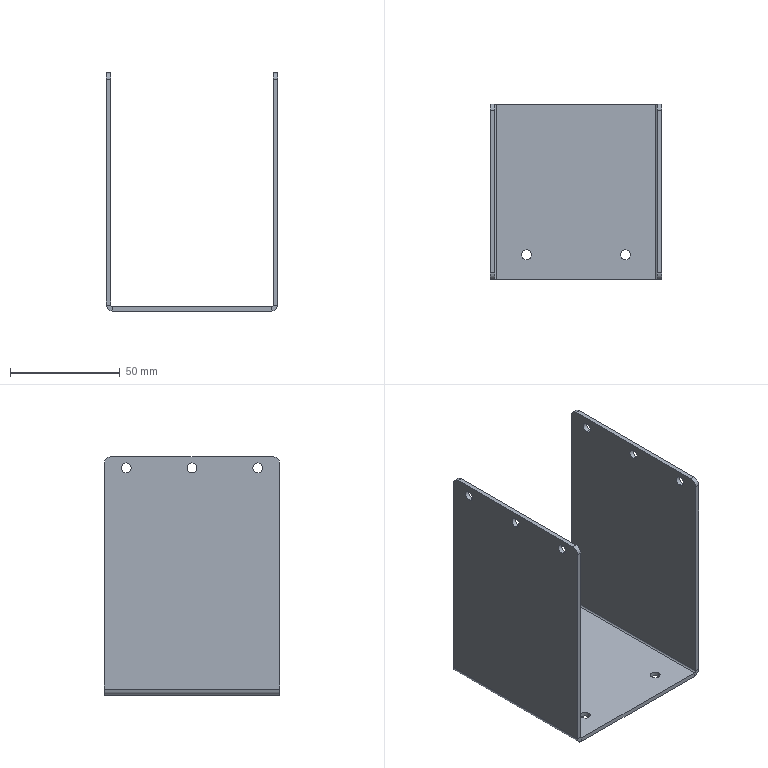Part | SolidWorks | features HoleWzd 2, Fillet 1, FlatPattern 1, SMBaseFlange 1, SheetMetal 1 | 1 solid | 42 faces | box 78 x 80 x 108.5 mm | volume 46050 mm3 | cylinder 24 | plane 18 | commonest cylinder face diameters 4.5 x16 6 x4 1.5 x2 5.5 x2
STEP:
#1=CARTESIAN_POINT('',(78.,10.,-7.25));
#2=VERTEX_POINT('',#1);
#3=CARTESIAN_POINT('',(78.,10.,-2.75));
#4=VERTEX_POINT('',#3);
#5=CARTESIAN_POINT('',(78.,10.,-5.));
#6=DIRECTION('',(-1.,0.,0.));
#7=DIRECTION('',(0.,0.,1.));
#8=AXIS2_PLACEMENT_3D('',#5,#6,#7);
#9=CIRCLE('',#8,2.25);
#10=EDGE_CURVE('',#2,#4,#9,.T.);
#11=ORIENTED_EDGE('',*,*,#10,.F.);
#12=CARTESIAN_POINT('',(76.,10.,-7.25));
#13=VERTEX_POINT('',#12);
#14=CARTESIAN_POINT('',(0.,10.,-7.25));
#15=DIRECTION('',(-1.,0.,0.));
#16=VECTOR('',#15,1000.);
#17=LINE('',#14,#16);
#18=EDGE_CURVE('',#2,#13,#17,.T.);
#19=ORIENTED_EDGE('',*,*,#18,.T.);
#20=CARTESIAN_POINT('',(76.,10.,-2.75));
#21=VERTEX_POINT('',#20);
#22=CARTESIAN_POINT('',(76.,10.,-5.));
#23=DIRECTION('',(1.,0.,0.));
#24=DIRECTION('',(0.,0.,-1.));
#25=AXIS2_PLACEMENT_3D('',#22,#23,#24);
#26=CIRCLE('',#25,2.25);
#27=EDGE_CURVE('',#21,#13,#26,.T.);
#28=ORIENTED_EDGE('',*,*,#27,.F.);
#29=CARTESIAN_POINT('',(0.,10.,-2.75));
#30=DIRECTION('',(-1.,0.,0.));
#31=VECTOR('',#30,1000.);
#32=LINE('',#29,#31);
#33=EDGE_CURVE('',#4,#21,#32,.T.);
#34=ORIENTED_EDGE('',*,*,#33,.F.);
#35=EDGE_LOOP('',(#11,#19,#28,#34));
#36=FACE_OUTER_BOUND('',#35,.T.);
#37=CARTESIAN_POINT('',(0.,10.,-5.));
#38=DIRECTION('',(-1.,0.,0.));
#39=DIRECTION('',(0.,0.,1.));
#40=AXIS2_PLACEMENT_3D('',#37,#38,#39);
#41=CYLINDRICAL_SURFACE('',#40,2.25);
#42=ADVANCED_FACE('',(#36),#41,.F.);
#43=CARTESIAN_POINT('',(2.,10.,-7.25));
#44=VERTEX_POINT('',#43);
#45=CARTESIAN_POINT('',(2.,10.,-2.75));
#46=VERTEX_POINT('',#45);
#47=CARTESIAN_POINT('',(2.,10.,-5.));
#48=DIRECTION('',(-1.,0.,0.));
#49=DIRECTION('',(0.,0.,1.));
#50=AXIS2_PLACEMENT_3D('',#47,#48,#49);
#51=CIRCLE('',#50,2.25);
#52=EDGE_CURVE('',#44,#46,#51,.T.);
#53=ORIENTED_EDGE('',*,*,#52,.F.);
#54=CARTESIAN_POINT('',(0.,10.,-7.25));
#55=VERTEX_POINT('',#54);
#56=CARTESIAN_POINT('',(0.,10.,-7.25));
#57=DIRECTION('',(-1.,0.,0.));
#58=VECTOR('',#57,1000.);
#59=LINE('',#56,#58);
#60=EDGE_CURVE('',#44,#55,#59,.T.);
#61=ORIENTED_EDGE('',*,*,#60,.T.);
#62=CARTESIAN_POINT('',(0.,10.,-2.75));
#63=VERTEX_POINT('',#62);
#64=CARTESIAN_POINT('',(0.,10.,-5.));
#65=DIRECTION('',(-1.,0.,0.));
#66=DIRECTION('',(0.,0.,1.));
#67=AXIS2_PLACEMENT_3D('',#64,#65,#66);
#68=CIRCLE('',#67,2.25);
#69=EDGE_CURVE('',#55,#63,#68,.T.);
#70=ORIENTED_EDGE('',*,*,#69,.T.);
#71=CARTESIAN_POINT('',(0.,10.,-2.75));
#72=DIRECTION('',(-1.,0.,0.));
#73=VECTOR('',#72,1000.);
#74=LINE('',#71,#73);
#75=EDGE_CURVE('',#46,#63,#74,.T.);
#76=ORIENTED_EDGE('',*,*,#75,.F.);
#77=EDGE_LOOP('',(#53,#61,#70,#76));
#78=FACE_OUTER_BOUND('',#77,.T.);
#79=CARTESIAN_POINT('',(0.,10.,-5.));
#80=DIRECTION('',(-1.,0.,0.));
#81=DIRECTION('',(0.,0.,1.));
#82=AXIS2_PLACEMENT_3D('',#79,#80,#81);
#83=CYLINDRICAL_SURFACE('',#82,2.25);
#84=ADVANCED_FACE('',(#78),#83,.F.);
#85=CARTESIAN_POINT('',(2.,40.,-7.25));
#86=VERTEX_POINT('',#85);
#87=CARTESIAN_POINT('',(2.,40.,-2.75));
#88=VERTEX_POINT('',#87);
#89=CARTESIAN_POINT('',(2.,40.,-5.));
#90=DIRECTION('',(-1.,0.,0.));
#91=DIRECTION('',(0.,0.,1.));
#92=AXIS2_PLACEMENT_3D('',#89,#90,#91);
#93=CIRCLE('',#92,2.25);
#94=EDGE_CURVE('',#86,#88,#93,.T.);
#95=ORIENTED_EDGE('',*,*,#94,.F.);
#96=CARTESIAN_POINT('',(0.,40.,-7.25));
#97=VERTEX_POINT('',#96);
#98=CARTESIAN_POINT('',(0.,40.,-7.25));
#99=DIRECTION('',(-1.,0.,0.));
#100=VECTOR('',#99,1000.);
#101=LINE('',#98,#100);
#102=EDGE_CURVE('',#86,#97,#101,.T.);
#103=ORIENTED_EDGE('',*,*,#102,.T.);
#104=CARTESIAN_POINT('',(0.,40.,-2.75));
#105=VERTEX_POINT('',#104);
#106=CARTESIAN_POINT('',(0.,40.,-5.));
#107=DIRECTION('',(-1.,0.,0.));
#108=DIRECTION('',(0.,0.,1.));
#109=AXIS2_PLACEMENT_3D('',#106,#107,#108);
#110=CIRCLE('',#109,2.25);
#111=EDGE_CURVE('',#97,#105,#110,.T.);
#112=ORIENTED_EDGE('',*,*,#111,.T.);
#113=CARTESIAN_POINT('',(0.,40.,-2.75));
#114=DIRECTION('',(-1.,0.,0.));
#115=VECTOR('',#114,1000.);
#116=LINE('',#113,#115);
#117=EDGE_CURVE('',#88,#105,#116,.T.);
#118=ORIENTED_EDGE('',*,*,#117,.F.);
#119=EDGE_LOOP('',(#95,#103,#112,#118));
#120=FACE_OUTER_BOUND('',#119,.T.);
#121=CARTESIAN_POINT('',(0.,40.,-5.));
#122=DIRECTION('',(-1.,0.,0.));
#123=DIRECTION('',(0.,0.,1.));
#124=AXIS2_PLACEMENT_3D('',#121,#122,#123);
#125=CYLINDRICAL_SURFACE('',#124,2.25);
#126=ADVANCED_FACE('',(#120),#125,.F.);
#127=CARTESIAN_POINT('',(78.,40.,-7.25));
#128=VERTEX_POINT('',#127);
#129=CARTESIAN_POINT('',(78.,40.,-2.75));
#130=VERTEX_POINT('',#129);
#131=CARTESIAN_POINT('',(78.,40.,-5.));
#132=DIRECTION('',(-1.,0.,0.));
#133=DIRECTION('',(0.,0.,1.));
#134=AXIS2_PLACEMENT_3D('',#131,#132,#133);
#135=CIRCLE('',#134,2.25);
#136=EDGE_CURVE('',#128,#130,#135,.T.);
#137=ORIENTED_EDGE('',*,*,#136,.F.);
#138=CARTESIAN_POINT('',(76.,40.,-7.25));
#139=VERTEX_POINT('',#138);
#140=CARTESIAN_POINT('',(0.,40.,-7.25));
#141=DIRECTION('',(-1.,0.,0.));
#142=VECTOR('',#141,1000.);
#143=LINE('',#140,#142);
#144=EDGE_CURVE('',#128,#139,#143,.T.);
#145=ORIENTED_EDGE('',*,*,#144,.T.);
#146=CARTESIAN_POINT('',(76.,40.,-2.75));
#147=VERTEX_POINT('',#146);
#148=CARTESIAN_POINT('',(76.,40.,-5.));
#149=DIRECTION('',(1.,0.,0.));
#150=DIRECTION('',(0.,0.,-1.));
#151=AXIS2_PLACEMENT_3D('',#148,#149,#150);
#152=CIRCLE('',#151,2.25);
#153=EDGE_CURVE('',#147,#139,#152,.T.);
#154=ORIENTED_EDGE('',*,*,#153,.F.);
#155=CARTESIAN_POINT('',(0.,40.,-2.75));
#156=DIRECTION('',(-1.,0.,0.));
#157=VECTOR('',#156,1000.);
#158=LINE('',#155,#157);
#159=EDGE_CURVE('',#130,#147,#158,.T.);
#160=ORIENTED_EDGE('',*,*,#159,.F.);
#161=EDGE_LOOP('',(#137,#145,#154,#160));
#162=FACE_OUTER_BOUND('',#161,.T.);
#163=CARTESIAN_POINT('',(0.,40.,-5.));
#164=DIRECTION('',(-1.,0.,0.));
#165=DIRECTION('',(0.,0.,1.));
#166=AXIS2_PLACEMENT_3D('',#163,#164,#165);
#167=CYLINDRICAL_SURFACE('',#166,2.25);
#168=ADVANCED_FACE('',(#162),#167,.F.);
#169=CARTESIAN_POINT('',(2.,70.,-7.25));
#170=VERTEX_POINT('',#169);
#171=CARTESIAN_POINT('',(2.,70.,-2.75));
#172=VERTEX_POINT('',#171);
#173=CARTESIAN_POINT('',(2.,70.,-5.));
#174=DIRECTION('',(-1.,0.,0.));
#175=DIRECTION('',(0.,0.,1.));
#176=AXIS2_PLACEMENT_3D('',#173,#174,#175);
#177=CIRCLE('',#176,2.25);
#178=EDGE_CURVE('',#170,#172,#177,.T.);
#179=ORIENTED_EDGE('',*,*,#178,.F.);
#180=CARTESIAN_POINT('',(0.,70.,-7.25));
#181=VERTEX_POINT('',#180);
#182=CARTESIAN_POINT('',(0.,70.,-7.25));
#183=DIRECTION('',(-1.,0.,0.));
#184=VECTOR('',#183,1000.);
#185=LINE('',#182,#184);
#186=EDGE_CURVE('',#170,#181,#185,.T.);
#187=ORIENTED_EDGE('',*,*,#186,.T.);
#188=CARTESIAN_POINT('',(0.,70.,-2.75));
#189=VERTEX_POINT('',#188);
#190=CARTESIAN_POINT('',(0.,70.,-5.));
#191=DIRECTION('',(-1.,0.,0.));
#192=DIRECTION('',(0.,0.,1.));
#193=AXIS2_PLACEMENT_3D('',#190,#191,#192);
#194=CIRCLE('',#193,2.25);
#195=EDGE_CURVE('',#181,#189,#194,.T.);
#196=ORIENTED_EDGE('',*,*,#195,.T.);
#197=CARTESIAN_POINT('',(0.,70.,-2.75));
#198=DIRECTION('',(-1.,0.,0.));
#199=VECTOR('',#198,1000.);
#200=LINE('',#197,#199);
#201=EDGE_CURVE('',#172,#189,#200,.T.);
#202=ORIENTED_EDGE('',*,*,#201,.F.);
#203=EDGE_LOOP('',(#179,#187,#196,#202));
#204=FACE_OUTER_BOUND('',#203,.T.);
#205=CARTESIAN_POINT('',(0.,70.,-5.));
#206=DIRECTION('',(-1.,0.,0.));
#207=DIRECTION('',(0.,0.,1.));
#208=AXIS2_PLACEMENT_3D('',#205,#206,#207);
#209=CYLINDRICAL_SURFACE('',#208,2.25);
#210=ADVANCED_FACE('',(#204),#209,.F.);
#211=CARTESIAN_POINT('',(78.,70.,-7.25));
#212=VERTEX_POINT('',#211);
#213=CARTESIAN_POINT('',(78.,70.,-2.75));
#214=VERTEX_POINT('',#213);
#215=CARTESIAN_POINT('',(78.,70.,-5.));
#216=DIRECTION('',(-1.,0.,0.));
#217=DIRECTION('',(0.,0.,1.));
#218=AXIS2_PLACEMENT_3D('',#215,#216,#217);
#219=CIRCLE('',#218,2.25);
#220=EDGE_CURVE('',#212,#214,#219,.T.);
#221=ORIENTED_EDGE('',*,*,#220,.F.);
#222=CARTESIAN_POINT('',(76.,70.,-7.25));
#223=VERTEX_POINT('',#222);
#224=CARTESIAN_POINT('',(0.,70.,-7.25));
#225=DIRECTION('',(-1.,0.,0.));
#226=VECTOR('',#225,1000.);
#227=LINE('',#224,#226);
#228=EDGE_CURVE('',#212,#223,#227,.T.);
#229=ORIENTED_EDGE('',*,*,#228,.T.);
#230=CARTESIAN_POINT('',(76.,70.,-2.75));
#231=VERTEX_POINT('',#230);
#232=CARTESIAN_POINT('',(76.,70.,-5.));
#233=DIRECTION('',(1.,0.,0.));
#234=DIRECTION('',(0.,0.,-1.));
#235=AXIS2_PLACEMENT_3D('',#232,#233,#234);
#236=CIRCLE('',#235,2.25);
#237=EDGE_CURVE('',#231,#223,#236,.T.);
#238=ORIENTED_EDGE('',*,*,#237,.F.);
#239=CARTESIAN_POINT('',(0.,70.,-2.75));
#240=DIRECTION('',(-1.,0.,0.));
#241=VECTOR('',#240,1000.);
#242=LINE('',#239,#241);
#243=EDGE_CURVE('',#214,#231,#242,.T.);
#244=ORIENTED_EDGE('',*,*,#243,.F.);
#245=EDGE_LOOP('',(#221,#229,#238,#244));
#246=FACE_OUTER_BOUND('',#245,.T.);
#247=CARTESIAN_POINT('',(0.,70.,-5.));
#248=DIRECTION('',(-1.,0.,0.));
#249=DIRECTION('',(0.,0.,1.));
#250=AXIS2_PLACEMENT_3D('',#247,#248,#249);
#251=CYLINDRICAL_SURFACE('',#250,2.25);
#252=ADVANCED_FACE('',(#246),#251,.F.);
#253=CARTESIAN_POINT('',(63.75,11.5,-106.5));
#254=VERTEX_POINT('',#253);
#255=CARTESIAN_POINT('',(59.25,11.5,-106.5));
#256=VERTEX_POINT('',#255);
#257=CARTESIAN_POINT('',(61.5,11.5,-106.5));
#258=DIRECTION('',(0.,0.,-1.));
#259=DIRECTION('',(-1.,0.,0.));
#260=AXIS2_PLACEMENT_3D('',#257,#258,#259);
#261=CIRCLE('',#260,2.25);
#262=EDGE_CURVE('',#254,#256,#261,.T.);
#263=ORIENTED_EDGE('',*,*,#262,.F.);
#264=CARTESIAN_POINT('',(63.75,11.5,-108.5));
#265=VERTEX_POINT('',#264);
#266=CARTESIAN_POINT('',(63.75,11.5,-108.5));
#267=DIRECTION('',(0.,0.,-1.));
#268=VECTOR('',#267,1000.);
#269=LINE('',#266,#268);
#270=EDGE_CURVE('',#254,#265,#269,.T.);
#271=ORIENTED_EDGE('',*,*,#270,.T.);
#272=CARTESIAN_POINT('',(59.25,11.5,-108.5));
#273=VERTEX_POINT('',#272);
#274=CARTESIAN_POINT('',(61.5,11.5,-108.5));
#275=DIRECTION('',(0.,0.,-1.));
#276=DIRECTION('',(-1.,0.,0.));
#277=AXIS2_PLACEMENT_3D('',#274,#275,#276);
#278=CIRCLE('',#277,2.25);
#279=EDGE_CURVE('',#265,#273,#278,.T.);
#280=ORIENTED_EDGE('',*,*,#279,.T.);
#281=CARTESIAN_POINT('',(59.25,11.5,-108.5));
#282=DIRECTION('',(0.,0.,-1.));
#283=VECTOR('',#282,1000.);
#284=LINE('',#281,#283);
#285=EDGE_CURVE('',#256,#273,#284,.T.);
#286=ORIENTED_EDGE('',*,*,#285,.F.);
#287=EDGE_LOOP('',(#263,#271,#280,#286));
#288=FACE_OUTER_BOUND('',#287,.T.);
#289=CARTESIAN_POINT('',(61.5,11.5,-108.5));
#290=DIRECTION('',(0.,0.,-1.));
#291=DIRECTION('',(-1.,0.,0.));
#292=AXIS2_PLACEMENT_3D('',#289,#290,#291);
#293=CYLINDRICAL_SURFACE('',#292,2.25);
#294=ADVANCED_FACE('',(#288),#293,.F.);
#295=CARTESIAN_POINT('',(18.75,11.5,-106.5));
#296=VERTEX_POINT('',#295);
#297=CARTESIAN_POINT('',(14.25,11.5,-106.5));
#298=VERTEX_POINT('',#297);
#299=CARTESIAN_POINT('',(16.5,11.5,-106.5));
#300=DIRECTION('',(0.,0.,-1.));
#301=DIRECTION('',(-1.,0.,0.));
#302=AXIS2_PLACEMENT_3D('',#299,#300,#301);
#303=CIRCLE('',#302,2.25);
#304=EDGE_CURVE('',#296,#298,#303,.T.);
#305=ORIENTED_EDGE('',*,*,#304,.F.);
#306=CARTESIAN_POINT('',(18.75,11.5,-108.5));
#307=VERTEX_POINT('',#306);
#308=CARTESIAN_POINT('',(18.75,11.5,-108.5));
#309=DIRECTION('',(0.,0.,-1.));
#310=VECTOR('',#309,1000.);
#311=LINE('',#308,#310);
#312=EDGE_CURVE('',#296,#307,#311,.T.);
#313=ORIENTED_EDGE('',*,*,#312,.T.);
#314=CARTESIAN_POINT('',(14.25,11.5,-108.5));
#315=VERTEX_POINT('',#314);
#316=CARTESIAN_POINT('',(16.5,11.5,-108.5));
#317=DIRECTION('',(0.,0.,-1.));
#318=DIRECTION('',(-1.,0.,0.));
#319=AXIS2_PLACEMENT_3D('',#316,#317,#318);
#320=CIRCLE('',#319,2.25);
#321=EDGE_CURVE('',#307,#315,#320,.T.);
#322=ORIENTED_EDGE('',*,*,#321,.T.);
#323=CARTESIAN_POINT('',(14.25,11.5,-108.5));
#324=DIRECTION('',(0.,0.,-1.));
#325=VECTOR('',#324,1000.);
#326=LINE('',#323,#325);
#327=EDGE_CURVE('',#298,#315,#326,.T.);
#328=ORIENTED_EDGE('',*,*,#327,.F.);
#329=EDGE_LOOP('',(#305,#313,#322,#328));
#330=FACE_OUTER_BOUND('',#329,.T.);
#331=CARTESIAN_POINT('',(16.5,11.5,-108.5));
#332=DIRECTION('',(0.,0.,-1.));
#333=DIRECTION('',(-1.,0.,0.));
#334=AXIS2_PLACEMENT_3D('',#331,#332,#333);
#335=CYLINDRICAL_SURFACE('',#334,2.25);
#336=ADVANCED_FACE('',(#330),#335,.F.);
#337=CARTESIAN_POINT('',(2.75,80.,-108.5));
#338=VERTEX_POINT('',#337);
#339=CARTESIAN_POINT('',(2.75,80.,-106.5));
#340=VERTEX_POINT('',#339);
#341=CARTESIAN_POINT('',(2.75,80.,-108.5));
#342=DIRECTION('',(0.,0.,1.));
#343=VECTOR('',#342,1000.);
#344=LINE('',#341,#343);
#345=EDGE_CURVE('',#338,#340,#344,.T.);
#346=ORIENTED_EDGE('',*,*,#345,.F.);
#347=CARTESIAN_POINT('',(0.,80.,-105.75));
#348=VERTEX_POINT('',#347);
#349=CARTESIAN_POINT('',(2.75,80.,-105.75));
#350=DIRECTION('',(0.,-1.,0.));
#351=DIRECTION('',(0.,0.,1.));
#352=AXIS2_PLACEMENT_3D('',#349,#350,#351);
#353=CIRCLE('',#352,2.75);
#354=EDGE_CURVE('',#348,#338,#353,.T.);
#355=ORIENTED_EDGE('',*,*,#354,.F.);
#356=CARTESIAN_POINT('',(2.,80.,-105.75));
#357=VERTEX_POINT('',#356);
#358=CARTESIAN_POINT('',(2.,80.,-105.75));
#359=DIRECTION('',(-1.,0.,0.));
#360=VECTOR('',#359,1000.);
#361=LINE('',#358,#360);
#362=EDGE_CURVE('',#357,#348,#361,.T.);
#363=ORIENTED_EDGE('',*,*,#362,.F.);
#364=CARTESIAN_POINT('',(2.75,80.,-105.75));
#365=DIRECTION('',(0.,-1.,0.));
#366=DIRECTION('',(1.,0.,0.));
#367=AXIS2_PLACEMENT_3D('',#364,#365,#366);
#368=CIRCLE('',#367,0.75);
#369=EDGE_CURVE('',#357,#340,#368,.T.);
#370=ORIENTED_EDGE('',*,*,#369,.T.);
#371=EDGE_LOOP('',(#346,#355,#363,#370));
#372=FACE_OUTER_BOUND('',#371,.T.);
#373=CARTESIAN_POINT('',(2.75,80.,-108.5));
#374=DIRECTION('',(0.,1.,0.));
#375=DIRECTION('',(0.,0.,1.));
#376=AXIS2_PLACEMENT_3D('',#373,#374,#375);
#377=PLANE('',#376);
#378=ADVANCED_FACE('',(#372),#377,.T.);
#379=CARTESIAN_POINT('',(75.25,80.,-108.5));
#380=VERTEX_POINT('',#379);
#381=CARTESIAN_POINT('',(0.,80.,-108.5));
#382=DIRECTION('',(1.,0.,0.));
#383=VECTOR('',#382,1000.);
#384=LINE('',#381,#383);
#385=EDGE_CURVE('',#338,#380,#384,.T.);
#386=ORIENTED_EDGE('',*,*,#385,.F.);
#387=ORIENTED_EDGE('',*,*,#345,.T.);
#388=CARTESIAN_POINT('',(75.25,80.,-106.5));
#389=VERTEX_POINT('',#388);
#390=CARTESIAN_POINT('',(0.,80.,-106.5));
#391=DIRECTION('',(1.,0.,0.));
#392=VECTOR('',#391,1000.);
#393=LINE('',#390,#392);
#394=EDGE_CURVE('',#340,#389,#393,.T.);
#395=ORIENTED_EDGE('',*,*,#394,.T.);
#396=CARTESIAN_POINT('',(75.25,80.,-106.5));
#397=DIRECTION('',(0.,0.,-1.));
#398=VECTOR('',#397,1000.);
#399=LINE('',#396,#398);
#400=EDGE_CURVE('',#389,#380,#399,.T.);
#401=ORIENTED_EDGE('',*,*,#400,.T.);
#402=EDGE_LOOP('',(#386,#387,#395,#401));
#403=FACE_OUTER_BOUND('',#402,.T.);
#404=CARTESIAN_POINT('',(2.,80.,-105.75));
#405=DIRECTION('',(0.,1.,0.));
#406=DIRECTION('',(0.,0.,1.));
#407=AXIS2_PLACEMENT_3D('',#404,#405,#406);
#408=PLANE('',#407);
#409=ADVANCED_FACE('',(#403),#408,.T.);
#410=CARTESIAN_POINT('',(0.,0.,-105.75));
#411=VERTEX_POINT('',#410);
#412=CARTESIAN_POINT('',(2.,0.,-105.75));
#413=VERTEX_POINT('',#412);
#414=CARTESIAN_POINT('',(0.,0.,-105.75));
#415=DIRECTION('',(1.,0.,0.));
#416=VECTOR('',#415,1000.);
#417=LINE('',#414,#416);
#418=EDGE_CURVE('',#411,#413,#417,.T.);
#419=ORIENTED_EDGE('',*,*,#418,.F.);
#420=CARTESIAN_POINT('',(2.75,0.,-108.5));
#421=VERTEX_POINT('',#420);
#422=CARTESIAN_POINT('',(2.75,0.,-105.75));
#423=DIRECTION('',(0.,-1.,0.));
#424=DIRECTION('',(0.,0.,1.));
#425=AXIS2_PLACEMENT_3D('',#422,#423,#424);
#426=CIRCLE('',#425,2.75);
#427=EDGE_CURVE('',#411,#421,#426,.T.);
#428=ORIENTED_EDGE('',*,*,#427,.T.);
#429=CARTESIAN_POINT('',(2.75,0.,-106.5));
#430=VERTEX_POINT('',#429);
#431=CARTESIAN_POINT('',(2.75,0.,-106.5));
#432=DIRECTION('',(0.,0.,-1.));
#433=VECTOR('',#432,1000.);
#434=LINE('',#431,#433);
#435=EDGE_CURVE('',#430,#421,#434,.T.);
#436=ORIENTED_EDGE('',*,*,#435,.F.);
#437=CARTESIAN_POINT('',(2.75,0.,-105.75));
#438=DIRECTION('',(0.,-1.,0.));
#439=DIRECTION('',(1.,0.,0.));
#440=AXIS2_PLACEMENT_3D('',#437,#438,#439);
#441=CIRCLE('',#440,0.75);
#442=EDGE_CURVE('',#413,#430,#441,.T.);
#443=ORIENTED_EDGE('',*,*,#442,.F.);
#444=EDGE_LOOP('',(#419,#428,#436,#443));
#445=FACE_OUTER_BOUND('',#444,.T.);
#446=CARTESIAN_POINT('',(0.,0.,-105.75));
#447=DIRECTION('',(0.,-1.,0.));
#448=DIRECTION('',(0.,0.,-1.));
#449=AXIS2_PLACEMENT_3D('',#446,#447,#448);
#450=PLANE('',#449);
#451=ADVANCED_FACE('',(#445),#450,.T.);
#452=CARTESIAN_POINT('',(2.,0.,-3.));
#453=VERTEX_POINT('',#452);
#454=CARTESIAN_POINT('',(2.,0.,0.));
#455=DIRECTION('',(0.,0.,-1.));
#456=VECTOR('',#455,1000.);
#457=LINE('',#454,#456);
#458=EDGE_CURVE('',#453,#413,#457,.T.);
#459=ORIENTED_EDGE('',*,*,#458,.F.);
#460=CARTESIAN_POINT('',(0.,0.,-3.));
#461=VERTEX_POINT('',#460);
#462=CARTESIAN_POINT('',(2.75,0.,-3.));
#463=DIRECTION('',(-1.,0.,0.));
#464=VECTOR('',#463,1000.);
#465=LINE('',#462,#464);
#466=EDGE_CURVE('',#453,#461,#465,.T.);
#467=ORIENTED_EDGE('',*,*,#466,.T.);
#468=CARTESIAN_POINT('',(0.,0.,0.));
#469=DIRECTION('',(0.,0.,-1.));
#470=VECTOR('',#469,1000.);
#471=LINE('',#468,#470);
#472=EDGE_CURVE('',#461,#411,#471,.T.);
#473=ORIENTED_EDGE('',*,*,#472,.T.);
#474=ORIENTED_EDGE('',*,*,#418,.T.);
#475=EDGE_LOOP('',(#459,#467,#473,#474));
#476=FACE_OUTER_BOUND('',#475,.T.);
#477=CARTESIAN_POINT('',(2.75,0.,-106.5));
#478=DIRECTION('',(0.,-1.,0.));
#479=DIRECTION('',(0.,0.,-1.));
#480=AXIS2_PLACEMENT_3D('',#477,#478,#479);
#481=PLANE('',#480);
#482=ADVANCED_FACE('',(#476),#481,.T.);
#483=CARTESIAN_POINT('',(78.,80.,-105.75));
#484=VERTEX_POINT('',#483);
#485=CARTESIAN_POINT('',(76.,80.,-105.75));
#486=VERTEX_POINT('',#485);
#487=CARTESIAN_POINT('',(78.,80.,-105.75));
#488=DIRECTION('',(-1.,0.,0.));
#489=VECTOR('',#488,1000.);
#490=LINE('',#487,#489);
#491=EDGE_CURVE('',#484,#486,#490,.T.);
#492=ORIENTED_EDGE('',*,*,#491,.F.);
#493=CARTESIAN_POINT('',(75.25,80.,-105.75));
#494=DIRECTION('',(0.,-1.,0.));
#495=DIRECTION('',(0.,0.,1.));
#496=AXIS2_PLACEMENT_3D('',#493,#494,#495);
#497=CIRCLE('',#496,2.75);
#498=EDGE_CURVE('',#380,#484,#497,.T.);
#499=ORIENTED_EDGE('',*,*,#498,.F.);
#500=ORIENTED_EDGE('',*,*,#400,.F.);
#501=CARTESIAN_POINT('',(75.25,80.,-105.75));
#502=DIRECTION('',(0.,-1.,0.));
#503=DIRECTION('',(1.,0.,0.));
#504=AXIS2_PLACEMENT_3D('',#501,#502,#503);
#505=CIRCLE('',#504,0.75);
#506=EDGE_CURVE('',#389,#486,#505,.T.);
#507=ORIENTED_EDGE('',*,*,#506,.T.);
#508=EDGE_LOOP('',(#492,#499,#500,#507));
#509=FACE_OUTER_BOUND('',#508,.T.);
#510=CARTESIAN_POINT('',(78.,80.,-105.75));
#511=DIRECTION('',(0.,1.,0.));
#512=DIRECTION('',(0.,0.,1.));
#513=AXIS2_PLACEMENT_3D('',#510,#511,#512);
#514=PLANE('',#513);
#515=ADVANCED_FACE('',(#509),#514,.T.);
#516=CARTESIAN_POINT('',(76.,80.,-3.));
#517=VERTEX_POINT('',#516);
#518=CARTESIAN_POINT('',(76.,80.,-108.5));
#519=DIRECTION('',(0.,0.,1.));
#520=VECTOR('',#519,1000.);
#521=LINE('',#518,#520);
#522=EDGE_CURVE('',#486,#517,#521,.T.);
#523=ORIENTED_EDGE('',*,*,#522,.T.);
#524=CARTESIAN_POINT('',(78.,80.,-3.));
#525=VERTEX_POINT('',#524);
#526=CARTESIAN_POINT('',(75.25,80.,-3.));
#527=DIRECTION('',(1.,0.,0.));
#528=VECTOR('',#527,1000.);
#529=LINE('',#526,#528);
#530=EDGE_CURVE('',#517,#525,#529,.T.);
#531=ORIENTED_EDGE('',*,*,#530,.T.);
#532=CARTESIAN_POINT('',(78.,80.,-108.5));
#533=DIRECTION('',(0.,0.,1.));
#534=VECTOR('',#533,1000.);
#535=LINE('',#532,#534);
#536=EDGE_CURVE('',#484,#525,#535,.T.);
#537=ORIENTED_EDGE('',*,*,#536,.F.);
#538=ORIENTED_EDGE('',*,*,#491,.T.);
#539=EDGE_LOOP('',(#523,#531,#537,#538));
#540=FACE_OUTER_BOUND('',#539,.T.);
#541=CARTESIAN_POINT('',(75.25,80.,-106.5));
#542=DIRECTION('',(0.,1.,0.));
#543=DIRECTION('',(0.,0.,1.));
#544=AXIS2_PLACEMENT_3D('',#541,#542,#543);
#545=PLANE('',#544);
#546=ADVANCED_FACE('',(#540),#545,.T.);
#547=CARTESIAN_POINT('',(75.25,0.,-108.5));
#548=VERTEX_POINT('',#547);
#549=CARTESIAN_POINT('',(75.25,0.,-106.5));
#550=VERTEX_POINT('',#549);
#551=CARTESIAN_POINT('',(75.25,0.,-108.5));
#552=DIRECTION('',(0.,0.,1.));
#553=VECTOR('',#552,1000.);
#554=LINE('',#551,#553);
#555=EDGE_CURVE('',#548,#550,#554,.T.);
#556=ORIENTED_EDGE('',*,*,#555,.F.);
#557=CARTESIAN_POINT('',(78.,0.,-105.75));
#558=VERTEX_POINT('',#557);
#559=CARTESIAN_POINT('',(75.25,0.,-105.75));
#560=DIRECTION('',(0.,-1.,0.));
#561=DIRECTION('',(0.,0.,1.));
#562=AXIS2_PLACEMENT_3D('',#559,#560,#561);
#563=CIRCLE('',#562,2.75);
#564=EDGE_CURVE('',#548,#558,#563,.T.);
#565=ORIENTED_EDGE('',*,*,#564,.T.);
#566=CARTESIAN_POINT('',(76.,0.,-105.75));
#567=VERTEX_POINT('',#566);
#568=CARTESIAN_POINT('',(76.,0.,-105.75));
#569=DIRECTION('',(1.,0.,0.));
#570=VECTOR('',#569,1000.);
#571=LINE('',#568,#570);
#572=EDGE_CURVE('',#567,#558,#571,.T.);
#573=ORIENTED_EDGE('',*,*,#572,.F.);
#574=CARTESIAN_POINT('',(75.25,0.,-105.75));
#575=DIRECTION('',(0.,-1.,0.));
#576=DIRECTION('',(1.,0.,0.));
#577=AXIS2_PLACEMENT_3D('',#574,#575,#576);
#578=CIRCLE('',#577,0.75);
#579=EDGE_CURVE('',#550,#567,#578,.T.);
#580=ORIENTED_EDGE('',*,*,#579,.F.);
#581=EDGE_LOOP('',(#556,#565,#573,#580));
#582=FACE_OUTER_BOUND('',#581,.T.);
#583=CARTESIAN_POINT('',(75.25,0.,-108.5));
#584=DIRECTION('',(0.,-1.,0.));
#585=DIRECTION('',(0.,0.,-1.));
#586=AXIS2_PLACEMENT_3D('',#583,#584,#585);
#587=PLANE('',#586);
#588=ADVANCED_FACE('',(#582),#587,.T.);
#589=CARTESIAN_POINT('',(0.,0.,-108.5));
#590=DIRECTION('',(1.,0.,0.));
#591=VECTOR('',#590,1000.);
#592=LINE('',#589,#591);
#593=EDGE_CURVE('',#421,#548,#592,.T.);
#594=ORIENTED_EDGE('',*,*,#593,.T.);
#595=ORIENTED_EDGE('',*,*,#555,.T.);
#596=CARTESIAN_POINT('',(0.,0.,-106.5));
#597=DIRECTION('',(1.,0.,0.));
#598=VECTOR('',#597,1000.);
#599=LINE('',#596,#598);
#600=EDGE_CURVE('',#430,#550,#599,.T.);
#601=ORIENTED_EDGE('',*,*,#600,.F.);
#602=ORIENTED_EDGE('',*,*,#435,.T.);
#603=EDGE_LOOP('',(#594,#595,#601,#602));
#604=FACE_OUTER_BOUND('',#603,.T.);
#605=CARTESIAN_POINT('',(76.,0.,-105.75));
#606=DIRECTION('',(0.,-1.,0.));
#607=DIRECTION('',(0.,0.,-1.));
#608=AXIS2_PLACEMENT_3D('',#605,#606,#607);
#609=PLANE('',#608);
#610=ADVANCED_FACE('',(#604),#609,.T.);
#611=ORIENTED_EDGE('',*,*,#27,.T.);
#612=CARTESIAN_POINT('',(76.,10.,-5.));
#613=DIRECTION('',(1.,0.,0.));
#614=DIRECTION('',(0.,0.,-1.));
#615=AXIS2_PLACEMENT_3D('',#612,#613,#614);
#616=CIRCLE('',#615,2.25);
#617=EDGE_CURVE('',#13,#21,#616,.T.);
#618=ORIENTED_EDGE('',*,*,#617,.T.);
#619=EDGE_LOOP('',(#611,#618));
#620=FACE_BOUND('',#619,.T.);
#621=ORIENTED_EDGE('',*,*,#153,.T.);
#622=CARTESIAN_POINT('',(76.,40.,-5.));
#623=DIRECTION('',(1.,0.,0.));
#624=DIRECTION('',(0.,0.,-1.));
#625=AXIS2_PLACEMENT_3D('',#622,#623,#624);
#626=CIRCLE('',#625,2.25);
#627=EDGE_CURVE('',#139,#147,#626,.T.);
#628=ORIENTED_EDGE('',*,*,#627,.T.);
#629=EDGE_LOOP('',(#621,#628));
#630=FACE_BOUND('',#629,.T.);
#631=ORIENTED_EDGE('',*,*,#237,.T.);
#632=CARTESIAN_POINT('',(76.,70.,-5.));
#633=DIRECTION('',(1.,0.,0.));
#634=DIRECTION('',(0.,0.,-1.));
#635=AXIS2_PLACEMENT_3D('',#632,#633,#634);
#636=CIRCLE('',#635,2.25);
#637=EDGE_CURVE('',#223,#231,#636,.T.);
#638=ORIENTED_EDGE('',*,*,#637,.T.);
#639=EDGE_LOOP('',(#631,#638));
#640=FACE_BOUND('',#639,.T.);
#641=CARTESIAN_POINT('',(76.,0.,-3.));
#642=VERTEX_POINT('',#641);
#643=CARTESIAN_POINT('',(76.,0.,-108.5));
#644=DIRECTION('',(0.,0.,1.));
#645=VECTOR('',#644,1000.);
#646=LINE('',#643,#645);
#647=EDGE_CURVE('',#567,#642,#646,.T.);
#648=ORIENTED_EDGE('',*,*,#647,.T.);
#649=CARTESIAN_POINT('',(76.,3.,0.));
#650=VERTEX_POINT('',#649);
#651=CARTESIAN_POINT('',(76.,3.,-3.));
#652=DIRECTION('',(-1.,0.,0.));
#653=DIRECTION('',(0.,0.,-1.));
#654=AXIS2_PLACEMENT_3D('',#651,#652,#653);
#655=CIRCLE('',#654,3.);
#656=EDGE_CURVE('',#642,#650,#655,.T.);
#657=ORIENTED_EDGE('',*,*,#656,.T.);
#658=CARTESIAN_POINT('',(76.,77.,0.));
#659=VERTEX_POINT('',#658);
#660=CARTESIAN_POINT('',(76.,80.,0.));
#661=DIRECTION('',(0.,-1.,0.));
#662=VECTOR('',#661,1000.);
#663=LINE('',#660,#662);
#664=EDGE_CURVE('',#659,#650,#663,.T.);
#665=ORIENTED_EDGE('',*,*,#664,.F.);
#666=CARTESIAN_POINT('',(76.,77.,-3.));
#667=DIRECTION('',(-1.,0.,0.));
#668=DIRECTION('',(0.,0.,-1.));
#669=AXIS2_PLACEMENT_3D('',#666,#667,#668);
#670=CIRCLE('',#669,3.);
#671=EDGE_CURVE('',#659,#517,#670,.T.);
#672=ORIENTED_EDGE('',*,*,#671,.T.);
#673=ORIENTED_EDGE('',*,*,#522,.F.);
#674=CARTESIAN_POINT('',(76.,80.,-105.75));
#675=DIRECTION('',(0.,-1.,0.));
#676=VECTOR('',#675,1000.);
#677=LINE('',#674,#676);
#678=EDGE_CURVE('',#486,#567,#677,.T.);
#679=ORIENTED_EDGE('',*,*,#678,.T.);
#680=EDGE_LOOP('',(#648,#657,#665,#672,#673,#679));
#681=FACE_OUTER_BOUND('',#680,.T.);
#682=CARTESIAN_POINT('',(76.,80.,-108.5));
#683=DIRECTION('',(1.,0.,0.));
#684=DIRECTION('',(0.,0.,-1.));
#685=AXIS2_PLACEMENT_3D('',#682,#683,#684);
#686=PLANE('',#685);
#687=ADVANCED_FACE('',(#620,#630,#640,#681),#686,.F.);
#688=ORIENTED_EDGE('',*,*,#664,.T.);
#689=CARTESIAN_POINT('',(78.,3.,0.));
#690=VERTEX_POINT('',#689);
#691=CARTESIAN_POINT('',(78.,3.,0.));
#692=DIRECTION('',(1.,0.,0.));
#693=VECTOR('',#692,1000.);
#694=LINE('',#691,#693);
#695=EDGE_CURVE('',#650,#690,#694,.T.);
#696=ORIENTED_EDGE('',*,*,#695,.T.);
#697=CARTESIAN_POINT('',(78.,77.,0.));
#698=VERTEX_POINT('',#697);
#699=CARTESIAN_POINT('',(78.,80.,0.));
#700=DIRECTION('',(0.,-1.,0.));
#701=VECTOR('',#700,1000.);
#702=LINE('',#699,#701);
#703=EDGE_CURVE('',#698,#690,#702,.T.);
#704=ORIENTED_EDGE('',*,*,#703,.F.);
#705=CARTESIAN_POINT('',(78.,77.,0.));
#706=DIRECTION('',(-1.,0.,0.));
#707=VECTOR('',#706,1000.);
#708=LINE('',#705,#707);
#709=EDGE_CURVE('',#698,#659,#708,.T.);
#710=ORIENTED_EDGE('',*,*,#709,.T.);
#711=EDGE_LOOP('',(#688,#696,#704,#710));
#712=FACE_OUTER_BOUND('',#711,.T.);
#713=CARTESIAN_POINT('',(78.,80.,0.));
#714=DIRECTION('',(0.,0.,1.));
#715=DIRECTION('',(1.,0.,0.));
#716=AXIS2_PLACEMENT_3D('',#713,#714,#715);
#717=PLANE('',#716);
#718=ADVANCED_FACE('',(#712),#717,.T.);
#719=CARTESIAN_POINT('',(78.,10.,-5.));
#720=DIRECTION('',(-1.,0.,0.));
#721=DIRECTION('',(0.,0.,1.));
#722=AXIS2_PLACEMENT_3D('',#719,#720,#721);
#723=CIRCLE('',#722,2.25);
#724=EDGE_CURVE('',#4,#2,#723,.T.);
#725=ORIENTED_EDGE('',*,*,#724,.T.);
#726=ORIENTED_EDGE('',*,*,#10,.T.);
#727=EDGE_LOOP('',(#725,#726));
#728=FACE_BOUND('',#727,.T.);
#729=CARTESIAN_POINT('',(78.,40.,-5.));
#730=DIRECTION('',(-1.,0.,0.));
#731=DIRECTION('',(0.,0.,1.));
#732=AXIS2_PLACEMENT_3D('',#729,#730,#731);
#733=CIRCLE('',#732,2.25);
#734=EDGE_CURVE('',#130,#128,#733,.T.);
#735=ORIENTED_EDGE('',*,*,#734,.T.);
#736=ORIENTED_EDGE('',*,*,#136,.T.);
#737=EDGE_LOOP('',(#735,#736));
#738=FACE_BOUND('',#737,.T.);
#739=CARTESIAN_POINT('',(78.,70.,-5.));
#740=DIRECTION('',(-1.,0.,0.));
#741=DIRECTION('',(0.,0.,1.));
#742=AXIS2_PLACEMENT_3D('',#739,#740,#741);
#743=CIRCLE('',#742,2.25);
#744=EDGE_CURVE('',#214,#212,#743,.T.);
#745=ORIENTED_EDGE('',*,*,#744,.T.);
#746=ORIENTED_EDGE('',*,*,#220,.T.);
#747=EDGE_LOOP('',(#745,#746));
#748=FACE_BOUND('',#747,.T.);
#749=ORIENTED_EDGE('',*,*,#703,.T.);
#750=CARTESIAN_POINT('',(78.,0.,-3.));
#751=VERTEX_POINT('',#750);
#752=CARTESIAN_POINT('',(78.,3.,-3.));
#753=DIRECTION('',(1.,0.,0.));
#754=DIRECTION('',(0.,0.,-1.));
#755=AXIS2_PLACEMENT_3D('',#752,#753,#754);
#756=CIRCLE('',#755,3.);
#757=EDGE_CURVE('',#690,#751,#756,.T.);
#758=ORIENTED_EDGE('',*,*,#757,.T.);
#759=CARTESIAN_POINT('',(78.,0.,-108.5));
#760=DIRECTION('',(0.,0.,1.));
#761=VECTOR('',#760,1000.);
#762=LINE('',#759,#761);
#763=EDGE_CURVE('',#558,#751,#762,.T.);
#764=ORIENTED_EDGE('',*,*,#763,.F.);
#765=CARTESIAN_POINT('',(78.,80.,-105.75));
#766=DIRECTION('',(0.,-1.,0.));
#767=VECTOR('',#766,1000.);
#768=LINE('',#765,#767);
#769=EDGE_CURVE('',#484,#558,#768,.T.);
#770=ORIENTED_EDGE('',*,*,#769,.F.);
#771=ORIENTED_EDGE('',*,*,#536,.T.);
#772=CARTESIAN_POINT('',(78.,77.,-3.));
#773=DIRECTION('',(1.,0.,0.));
#774=DIRECTION('',(0.,0.,-1.));
#775=AXIS2_PLACEMENT_3D('',#772,#773,#774);
#776=CIRCLE('',#775,3.);
#777=EDGE_CURVE('',#525,#698,#776,.T.);
#778=ORIENTED_EDGE('',*,*,#777,.T.);
#779=EDGE_LOOP('',(#749,#758,#764,#770,#771,#778));
#780=FACE_OUTER_BOUND('',#779,.T.);
#781=CARTESIAN_POINT('',(78.,80.,-108.5));
#782=DIRECTION('',(1.,0.,0.));
#783=DIRECTION('',(0.,0.,-1.));
#784=AXIS2_PLACEMENT_3D('',#781,#782,#783);
#785=PLANE('',#784);
#786=ADVANCED_FACE('',(#728,#738,#748,#780),#785,.T.);
#787=ORIENTED_EDGE('',*,*,#564,.F.);
#788=CARTESIAN_POINT('',(75.25,80.,-108.5));
#789=DIRECTION('',(0.,-1.,0.));
#790=VECTOR('',#789,1000.);
#791=LINE('',#788,#790);
#792=EDGE_CURVE('',#380,#548,#791,.T.);
#793=ORIENTED_EDGE('',*,*,#792,.F.);
#794=ORIENTED_EDGE('',*,*,#498,.T.);
#795=ORIENTED_EDGE('',*,*,#769,.T.);
#796=EDGE_LOOP('',(#787,#793,#794,#795));
#797=FACE_OUTER_BOUND('',#796,.T.);
#798=CARTESIAN_POINT('',(75.25,80.,-105.75));
#799=DIRECTION('',(0.,-1.,0.));
#800=DIRECTION('',(0.,0.,-1.));
#801=AXIS2_PLACEMENT_3D('',#798,#799,#800);
#802=CYLINDRICAL_SURFACE('',#801,2.75);
#803=ADVANCED_FACE('',(#797),#802,.T.);
#804=CARTESIAN_POINT('',(61.5,11.5,-108.5));
#805=DIRECTION('',(0.,0.,-1.));
#806=DIRECTION('',(-1.,0.,0.));
#807=AXIS2_PLACEMENT_3D('',#804,#805,#806);
#808=CIRCLE('',#807,2.25);
#809=EDGE_CURVE('',#273,#265,#808,.T.);
#810=ORIENTED_EDGE('',*,*,#809,.F.);
#811=ORIENTED_EDGE('',*,*,#279,.F.);
#812=EDGE_LOOP('',(#810,#811));
#813=FACE_BOUND('',#812,.T.);
#814=CARTESIAN_POINT('',(16.5,11.5,-108.5));
#815=DIRECTION('',(0.,0.,-1.));
#816=DIRECTION('',(-1.,0.,0.));
#817=AXIS2_PLACEMENT_3D('',#814,#815,#816);
#818=CIRCLE('',#817,2.25);
#819=EDGE_CURVE('',#315,#307,#818,.T.);
#820=ORIENTED_EDGE('',*,*,#819,.F.);
#821=ORIENTED_EDGE('',*,*,#321,.F.);
#822=EDGE_LOOP('',(#820,#821));
#823=FACE_BOUND('',#822,.T.);
#824=ORIENTED_EDGE('',*,*,#593,.F.);
#825=CARTESIAN_POINT('',(2.75,80.,-108.5));
#826=DIRECTION('',(0.,-1.,0.));
#827=VECTOR('',#826,1000.);
#828=LINE('',#825,#827);
#829=EDGE_CURVE('',#338,#421,#828,.T.);
#830=ORIENTED_EDGE('',*,*,#829,.F.);
#831=ORIENTED_EDGE('',*,*,#385,.T.);
#832=ORIENTED_EDGE('',*,*,#792,.T.);
#833=EDGE_LOOP('',(#824,#830,#831,#832));
#834=FACE_OUTER_BOUND('',#833,.T.);
#835=CARTESIAN_POINT('',(0.,80.,-108.5));
#836=DIRECTION('',(0.,0.,-1.));
#837=DIRECTION('',(-1.,0.,0.));
#838=AXIS2_PLACEMENT_3D('',#835,#836,#837);
#839=PLANE('',#838);
#840=ADVANCED_FACE('',(#813,#823,#834),#839,.T.);
#841=ORIENTED_EDGE('',*,*,#427,.F.);
#842=CARTESIAN_POINT('',(0.,80.,-105.75));
#843=DIRECTION('',(0.,-1.,0.));
#844=VECTOR('',#843,1000.);
#845=LINE('',#842,#844);
#846=EDGE_CURVE('',#348,#411,#845,.T.);
#847=ORIENTED_EDGE('',*,*,#846,.F.);
#848=ORIENTED_EDGE('',*,*,#354,.T.);
#849=ORIENTED_EDGE('',*,*,#829,.T.);
#850=EDGE_LOOP('',(#841,#847,#848,#849));
#851=FACE_OUTER_BOUND('',#850,.T.);
#852=CARTESIAN_POINT('',(2.75,80.,-105.75));
#853=DIRECTION('',(0.,-1.,0.));
#854=DIRECTION('',(0.,0.,-1.));
#855=AXIS2_PLACEMENT_3D('',#852,#853,#854);
#856=CYLINDRICAL_SURFACE('',#855,2.75);
#857=ADVANCED_FACE('',(#851),#856,.T.);
#858=CARTESIAN_POINT('',(0.,10.,-5.));
#859=DIRECTION('',(-1.,0.,0.));
#860=DIRECTION('',(0.,0.,1.));
#861=AXIS2_PLACEMENT_3D('',#858,#859,#860);
#862=CIRCLE('',#861,2.25);
#863=EDGE_CURVE('',#63,#55,#862,.T.);
#864=ORIENTED_EDGE('',*,*,#863,.F.);
#865=ORIENTED_EDGE('',*,*,#69,.F.);
#866=EDGE_LOOP('',(#864,#865));
#867=FACE_BOUND('',#866,.T.);
#868=CARTESIAN_POINT('',(0.,40.,-5.));
#869=DIRECTION('',(-1.,0.,0.));
#870=DIRECTION('',(0.,0.,1.));
#871=AXIS2_PLACEMENT_3D('',#868,#869,#870);
#872=CIRCLE('',#871,2.25);
#873=EDGE_CURVE('',#105,#97,#872,.T.);
#874=ORIENTED_EDGE('',*,*,#873,.F.);
#875=ORIENTED_EDGE('',*,*,#111,.F.);
#876=EDGE_LOOP('',(#874,#875));
#877=FACE_BOUND('',#876,.T.);
#878=CARTESIAN_POINT('',(0.,70.,-5.));
#879=DIRECTION('',(-1.,0.,0.));
#880=DIRECTION('',(0.,0.,1.));
#881=AXIS2_PLACEMENT_3D('',#878,#879,#880);
#882=CIRCLE('',#881,2.25);
#883=EDGE_CURVE('',#189,#181,#882,.T.);
#884=ORIENTED_EDGE('',*,*,#883,.F.);
#885=ORIENTED_EDGE('',*,*,#195,.F.);
#886=EDGE_LOOP('',(#884,#885));
#887=FACE_BOUND('',#886,.T.);
#888=CARTESIAN_POINT('',(0.,77.,0.));
#889=VERTEX_POINT('',#888);
#890=CARTESIAN_POINT('',(0.,3.,0.));
#891=VERTEX_POINT('',#890);
#892=CARTESIAN_POINT('',(0.,80.,0.));
#893=DIRECTION('',(0.,-1.,0.));
#894=VECTOR('',#893,1000.);
#895=LINE('',#892,#894);
#896=EDGE_CURVE('',#889,#891,#895,.T.);
#897=ORIENTED_EDGE('',*,*,#896,.F.);
#898=CARTESIAN_POINT('',(0.,80.,-3.));
#899=VERTEX_POINT('',#898);
#900=CARTESIAN_POINT('',(0.,77.,-3.));
#901=DIRECTION('',(-1.,0.,0.));
#902=DIRECTION('',(0.,0.,1.));
#903=AXIS2_PLACEMENT_3D('',#900,#901,#902);
#904=CIRCLE('',#903,3.);
#905=EDGE_CURVE('',#889,#899,#904,.T.);
#906=ORIENTED_EDGE('',*,*,#905,.T.);
#907=CARTESIAN_POINT('',(0.,80.,0.));
#908=DIRECTION('',(0.,0.,-1.));
#909=VECTOR('',#908,1000.);
#910=LINE('',#907,#909);
#911=EDGE_CURVE('',#899,#348,#910,.T.);
#912=ORIENTED_EDGE('',*,*,#911,.T.);
#913=ORIENTED_EDGE('',*,*,#846,.T.);
#914=ORIENTED_EDGE('',*,*,#472,.F.);
#915=CARTESIAN_POINT('',(0.,3.,-3.));
#916=DIRECTION('',(-1.,0.,0.));
#917=DIRECTION('',(0.,0.,1.));
#918=AXIS2_PLACEMENT_3D('',#915,#916,#917);
#919=CIRCLE('',#918,3.);
#920=EDGE_CURVE('',#461,#891,#919,.T.);
#921=ORIENTED_EDGE('',*,*,#920,.T.);
#922=EDGE_LOOP('',(#897,#906,#912,#913,#914,#921));
#923=FACE_OUTER_BOUND('',#922,.T.);
#924=CARTESIAN_POINT('',(0.,80.,0.));
#925=DIRECTION('',(-1.,0.,0.));
#926=DIRECTION('',(0.,0.,1.));
#927=AXIS2_PLACEMENT_3D('',#924,#925,#926);
#928=PLANE('',#927);
#929=ADVANCED_FACE('',(#867,#877,#887,#923),#928,.T.);
#930=CARTESIAN_POINT('',(2.,77.,0.));
#931=VERTEX_POINT('',#930);
#932=CARTESIAN_POINT('',(2.,3.,0.));
#933=VERTEX_POINT('',#932);
#934=CARTESIAN_POINT('',(2.,80.,0.));
#935=DIRECTION('',(0.,-1.,0.));
#936=VECTOR('',#935,1000.);
#937=LINE('',#934,#936);
#938=EDGE_CURVE('',#931,#933,#937,.T.);
#939=ORIENTED_EDGE('',*,*,#938,.F.);
#940=CARTESIAN_POINT('',(2.,77.,0.));
#941=DIRECTION('',(-1.,0.,0.));
#942=VECTOR('',#941,1000.);
#943=LINE('',#940,#942);
#944=EDGE_CURVE('',#931,#889,#943,.T.);
#945=ORIENTED_EDGE('',*,*,#944,.T.);
#946=ORIENTED_EDGE('',*,*,#896,.T.);
#947=CARTESIAN_POINT('',(2.,3.,0.));
#948=DIRECTION('',(1.,0.,0.));
#949=VECTOR('',#948,1000.);
#950=LINE('',#947,#949);
#951=EDGE_CURVE('',#891,#933,#950,.T.);
#952=ORIENTED_EDGE('',*,*,#951,.T.);
#953=EDGE_LOOP('',(#939,#945,#946,#952));
#954=FACE_OUTER_BOUND('',#953,.T.);
#955=CARTESIAN_POINT('',(2.,80.,0.));
#956=DIRECTION('',(0.,0.,1.));
#957=DIRECTION('',(1.,0.,0.));
#958=AXIS2_PLACEMENT_3D('',#955,#956,#957);
#959=PLANE('',#958);
#960=ADVANCED_FACE('',(#954),#959,.T.);
#961=CARTESIAN_POINT('',(2.,10.,-5.));
#962=DIRECTION('',(-1.,0.,0.));
#963=DIRECTION('',(0.,0.,1.));
#964=AXIS2_PLACEMENT_3D('',#961,#962,#963);
#965=CIRCLE('',#964,2.25);
#966=EDGE_CURVE('',#46,#44,#965,.T.);
#967=ORIENTED_EDGE('',*,*,#966,.T.);
#968=ORIENTED_EDGE('',*,*,#52,.T.);
#969=EDGE_LOOP('',(#967,#968));
#970=FACE_BOUND('',#969,.T.);
#971=CARTESIAN_POINT('',(2.,40.,-5.));
#972=DIRECTION('',(-1.,0.,0.));
#973=DIRECTION('',(0.,0.,1.));
#974=AXIS2_PLACEMENT_3D('',#971,#972,#973);
#975=CIRCLE('',#974,2.25);
#976=EDGE_CURVE('',#88,#86,#975,.T.);
#977=ORIENTED_EDGE('',*,*,#976,.T.);
#978=ORIENTED_EDGE('',*,*,#94,.T.);
#979=EDGE_LOOP('',(#977,#978));
#980=FACE_BOUND('',#979,.T.);
#981=CARTESIAN_POINT('',(2.,70.,-5.));
#982=DIRECTION('',(-1.,0.,0.));
#983=DIRECTION('',(0.,0.,1.));
#984=AXIS2_PLACEMENT_3D('',#981,#982,#983);
#985=CIRCLE('',#984,2.25);
#986=EDGE_CURVE('',#172,#170,#985,.T.);
#987=ORIENTED_EDGE('',*,*,#986,.T.);
#988=ORIENTED_EDGE('',*,*,#178,.T.);
#989=EDGE_LOOP('',(#987,#988));
#990=FACE_BOUND('',#989,.T.);
#991=CARTESIAN_POINT('',(2.,80.,-3.));
#992=VERTEX_POINT('',#991);
#993=CARTESIAN_POINT('',(2.,80.,0.));
#994=DIRECTION('',(0.,0.,-1.));
#995=VECTOR('',#994,1000.);
#996=LINE('',#993,#995);
#997=EDGE_CURVE('',#992,#357,#996,.T.);
#998=ORIENTED_EDGE('',*,*,#997,.F.);
#999=CARTESIAN_POINT('',(2.,77.,-3.));
#1000=DIRECTION('',(1.,0.,0.));
#1001=DIRECTION('',(0.,0.,1.));
#1002=AXIS2_PLACEMENT_3D('',#999,#1000,#1001);
#1003=CIRCLE('',#1002,3.);
#1004=EDGE_CURVE('',#992,#931,#1003,.T.);
#1005=ORIENTED_EDGE('',*,*,#1004,.T.);
#1006=ORIENTED_EDGE('',*,*,#938,.T.);
#1007=CARTESIAN_POINT('',(2.,3.,-3.));
#1008=DIRECTION('',(1.,0.,0.));
#1009=DIRECTION('',(0.,0.,1.));
#1010=AXIS2_PLACEMENT_3D('',#1007,#1008,#1009);
#1011=CIRCLE('',#1010,3.);
#1012=EDGE_CURVE('',#933,#453,#1011,.T.);
#1013=ORIENTED_EDGE('',*,*,#1012,.T.);
#1014=ORIENTED_EDGE('',*,*,#458,.T.);
#1015=CARTESIAN_POINT('',(2.,80.,-105.75));
#1016=DIRECTION('',(0.,-1.,0.));
#1017=VECTOR('',#1016,1000.);
#1018=LINE('',#1015,#1017);
#1019=EDGE_CURVE('',#357,#413,#1018,.T.);
#1020=ORIENTED_EDGE('',*,*,#1019,.F.);
#1021=EDGE_LOOP('',(#998,#1005,#1006,#1013,#1014,#1020));
#1022=FACE_OUTER_BOUND('',#1021,.T.);
#1023=CARTESIAN_POINT('',(2.,80.,0.));
#1024=DIRECTION('',(-1.,0.,0.));
#1025=DIRECTION('',(0.,0.,1.));
#1026=AXIS2_PLACEMENT_3D('',#1023,#1024,#1025);
#1027=PLANE('',#1026);
#1028=ADVANCED_FACE('',(#970,#980,#990,#1022),#1027,.F.);
#1029=ORIENTED_EDGE('',*,*,#442,.T.);
#1030=CARTESIAN_POINT('',(2.75,80.,-106.5));
#1031=DIRECTION('',(0.,-1.,0.));
#1032=VECTOR('',#1031,1000.);
#1033=LINE('',#1030,#1032);
#1034=EDGE_CURVE('',#340,#430,#1033,.T.);
#1035=ORIENTED_EDGE('',*,*,#1034,.F.);
#1036=ORIENTED_EDGE('',*,*,#369,.F.);
#1037=ORIENTED_EDGE('',*,*,#1019,.T.);
#1038=EDGE_LOOP('',(#1029,#1035,#1036,#1037));
#1039=FACE_OUTER_BOUND('',#1038,.T.);
#1040=CARTESIAN_POINT('',(2.75,80.,-105.75));
#1041=DIRECTION('',(0.,-1.,0.));
#1042=DIRECTION('',(0.,0.,-1.));
#1043=AXIS2_PLACEMENT_3D('',#1040,#1041,#1042);
#1044=CYLINDRICAL_SURFACE('',#1043,0.75);
#1045=ADVANCED_FACE('',(#1039),#1044,.F.);
#1046=CARTESIAN_POINT('',(61.5,11.5,-106.5));
#1047=DIRECTION('',(0.,0.,-1.));
#1048=DIRECTION('',(-1.,0.,0.));
#1049=AXIS2_PLACEMENT_3D('',#1046,#1047,#1048);
#1050=CIRCLE('',#1049,2.25);
#1051=EDGE_CURVE('',#256,#254,#1050,.T.);
#1052=ORIENTED_EDGE('',*,*,#1051,.T.);
#1053=ORIENTED_EDGE('',*,*,#262,.T.);
#1054=EDGE_LOOP('',(#1052,#1053));
#1055=FACE_BOUND('',#1054,.T.);
#1056=CARTESIAN_POINT('',(16.5,11.5,-106.5));
#1057=DIRECTION('',(0.,0.,-1.));
#1058=DIRECTION('',(-1.,0.,0.));
#1059=AXIS2_PLACEMENT_3D('',#1056,#1057,#1058);
#1060=CIRCLE('',#1059,2.25);
#1061=EDGE_CURVE('',#298,#296,#1060,.T.);
#1062=ORIENTED_EDGE('',*,*,#1061,.T.);
#1063=ORIENTED_EDGE('',*,*,#304,.T.);
#1064=EDGE_LOOP('',(#1062,#1063));
#1065=FACE_BOUND('',#1064,.T.);
#1066=ORIENTED_EDGE('',*,*,#600,.T.);
#1067=CARTESIAN_POINT('',(75.25,80.,-106.5));
#1068=DIRECTION('',(0.,-1.,0.));
#1069=VECTOR('',#1068,1000.);
#1070=LINE('',#1067,#1069);
#1071=EDGE_CURVE('',#389,#550,#1070,.T.);
#1072=ORIENTED_EDGE('',*,*,#1071,.F.);
#1073=ORIENTED_EDGE('',*,*,#394,.F.);
#1074=ORIENTED_EDGE('',*,*,#1034,.T.);
#1075=EDGE_LOOP('',(#1066,#1072,#1073,#1074));
#1076=FACE_OUTER_BOUND('',#1075,.T.);
#1077=CARTESIAN_POINT('',(0.,80.,-106.5));
#1078=DIRECTION('',(0.,0.,-1.));
#1079=DIRECTION('',(-1.,0.,0.));
#1080=AXIS2_PLACEMENT_3D('',#1077,#1078,#1079);
#1081=PLANE('',#1080);
#1082=ADVANCED_FACE('',(#1055,#1065,#1076),#1081,.F.);
#1083=ORIENTED_EDGE('',*,*,#579,.T.);
#1084=ORIENTED_EDGE('',*,*,#678,.F.);
#1085=ORIENTED_EDGE('',*,*,#506,.F.);
#1086=ORIENTED_EDGE('',*,*,#1071,.T.);
#1087=EDGE_LOOP('',(#1083,#1084,#1085,#1086));
#1088=FACE_OUTER_BOUND('',#1087,.T.);
#1089=CARTESIAN_POINT('',(75.25,80.,-105.75));
#1090=DIRECTION('',(0.,-1.,0.));
#1091=DIRECTION('',(0.,0.,-1.));
#1092=AXIS2_PLACEMENT_3D('',#1089,#1090,#1091);
#1093=CYLINDRICAL_SURFACE('',#1092,0.75);
#1094=ADVANCED_FACE('',(#1088),#1093,.F.);
#1095=ORIENTED_EDGE('',*,*,#911,.F.);
#1096=CARTESIAN_POINT('',(75.25,80.,-3.));
#1097=DIRECTION('',(1.,0.,0.));
#1098=VECTOR('',#1097,1000.);
#1099=LINE('',#1096,#1098);
#1100=EDGE_CURVE('',#899,#992,#1099,.T.);
#1101=ORIENTED_EDGE('',*,*,#1100,.T.);
#1102=ORIENTED_EDGE('',*,*,#997,.T.);
#1103=ORIENTED_EDGE('',*,*,#362,.T.);
#1104=EDGE_LOOP('',(#1095,#1101,#1102,#1103));
#1105=FACE_OUTER_BOUND('',#1104,.T.);
#1106=CARTESIAN_POINT('',(75.25,80.,-105.75));
#1107=DIRECTION('',(0.,1.,0.));
#1108=DIRECTION('',(1.,0.,0.));
#1109=AXIS2_PLACEMENT_3D('',#1106,#1107,#1108);
#1110=PLANE('',#1109);
#1111=ADVANCED_FACE('',(#1105),#1110,.T.);
#1112=ORIENTED_EDGE('',*,*,#763,.T.);
#1113=CARTESIAN_POINT('',(76.,0.,-3.));
#1114=DIRECTION('',(-1.,0.,0.));
#1115=VECTOR('',#1114,1000.);
#1116=LINE('',#1113,#1115);
#1117=EDGE_CURVE('',#751,#642,#1116,.T.);
#1118=ORIENTED_EDGE('',*,*,#1117,.T.);
#1119=ORIENTED_EDGE('',*,*,#647,.F.);
#1120=ORIENTED_EDGE('',*,*,#572,.T.);
#1121=EDGE_LOOP('',(#1112,#1118,#1119,#1120));
#1122=FACE_OUTER_BOUND('',#1121,.T.);
#1123=CARTESIAN_POINT('',(75.25,0.,-105.75));
#1124=DIRECTION('',(0.,1.,0.));
#1125=DIRECTION('',(1.,0.,0.));
#1126=AXIS2_PLACEMENT_3D('',#1123,#1124,#1125);
#1127=PLANE('',#1126);
#1128=ADVANCED_FACE('',(#1122),#1127,.F.);
#1129=ORIENTED_EDGE('',*,*,#757,.F.);
#1130=ORIENTED_EDGE('',*,*,#695,.F.);
#1131=ORIENTED_EDGE('',*,*,#656,.F.);
#1132=ORIENTED_EDGE('',*,*,#1117,.F.);
#1133=EDGE_LOOP('',(#1129,#1130,#1131,#1132));
#1134=FACE_OUTER_BOUND('',#1133,.T.);
#1135=CARTESIAN_POINT('',(75.25,3.,-3.));
#1136=DIRECTION('',(1.,0.,0.));
#1137=DIRECTION('',(0.,0.,-1.));
#1138=AXIS2_PLACEMENT_3D('',#1135,#1136,#1137);
#1139=CYLINDRICAL_SURFACE('',#1138,3.);
#1140=ADVANCED_FACE('',(#1134),#1139,.T.);
#1141=ORIENTED_EDGE('',*,*,#777,.F.);
#1142=ORIENTED_EDGE('',*,*,#530,.F.);
#1143=ORIENTED_EDGE('',*,*,#671,.F.);
#1144=ORIENTED_EDGE('',*,*,#709,.F.);
#1145=EDGE_LOOP('',(#1141,#1142,#1143,#1144));
#1146=FACE_OUTER_BOUND('',#1145,.T.);
#1147=CARTESIAN_POINT('',(78.,77.,-3.));
#1148=DIRECTION('',(-1.,0.,0.));
#1149=DIRECTION('',(0.,0.,1.));
#1150=AXIS2_PLACEMENT_3D('',#1147,#1148,#1149);
#1151=CYLINDRICAL_SURFACE('',#1150,3.);
#1152=ADVANCED_FACE('',(#1146),#1151,.T.);
#1153=ORIENTED_EDGE('',*,*,#1004,.F.);
#1154=ORIENTED_EDGE('',*,*,#1100,.F.);
#1155=ORIENTED_EDGE('',*,*,#905,.F.);
#1156=ORIENTED_EDGE('',*,*,#944,.F.);
#1157=EDGE_LOOP('',(#1153,#1154,#1155,#1156));
#1158=FACE_OUTER_BOUND('',#1157,.T.);
#1159=CARTESIAN_POINT('',(2.,77.,-3.));
#1160=DIRECTION('',(-1.,0.,0.));
#1161=DIRECTION('',(0.,0.,1.));
#1162=AXIS2_PLACEMENT_3D('',#1159,#1160,#1161);
#1163=CYLINDRICAL_SURFACE('',#1162,3.);
#1164=ADVANCED_FACE('',(#1158),#1163,.T.);
#1165=ORIENTED_EDGE('',*,*,#1012,.F.);
#1166=ORIENTED_EDGE('',*,*,#951,.F.);
#1167=ORIENTED_EDGE('',*,*,#920,.F.);
#1168=ORIENTED_EDGE('',*,*,#466,.F.);
#1169=EDGE_LOOP('',(#1165,#1166,#1167,#1168));
#1170=FACE_OUTER_BOUND('',#1169,.T.);
#1171=CARTESIAN_POINT('',(2.75,3.,-3.));
#1172=DIRECTION('',(-1.,0.,0.));
#1173=DIRECTION('',(0.,0.,1.));
#1174=AXIS2_PLACEMENT_3D('',#1171,#1172,#1173);
#1175=CYLINDRICAL_SURFACE('',#1174,3.);
#1176=ADVANCED_FACE('',(#1170),#1175,.T.);
#1177=ORIENTED_EDGE('',*,*,#312,.F.);
#1178=ORIENTED_EDGE('',*,*,#1061,.F.);
#1179=ORIENTED_EDGE('',*,*,#327,.T.);
#1180=ORIENTED_EDGE('',*,*,#819,.T.);
#1181=EDGE_LOOP('',(#1177,#1178,#1179,#1180));
#1182=FACE_OUTER_BOUND('',#1181,.T.);
#1183=CARTESIAN_POINT('',(16.5,11.5,-108.5));
#1184=DIRECTION('',(0.,0.,-1.));
#1185=DIRECTION('',(-1.,0.,0.));
#1186=AXIS2_PLACEMENT_3D('',#1183,#1184,#1185);
#1187=CYLINDRICAL_SURFACE('',#1186,2.25);
#1188=ADVANCED_FACE('',(#1182),#1187,.F.);
#1189=ORIENTED_EDGE('',*,*,#270,.F.);
#1190=ORIENTED_EDGE('',*,*,#1051,.F.);
#1191=ORIENTED_EDGE('',*,*,#285,.T.);
#1192=ORIENTED_EDGE('',*,*,#809,.T.);
#1193=EDGE_LOOP('',(#1189,#1190,#1191,#1192));
#1194=FACE_OUTER_BOUND('',#1193,.T.);
#1195=CARTESIAN_POINT('',(61.5,11.5,-108.5));
#1196=DIRECTION('',(0.,0.,-1.));
#1197=DIRECTION('',(-1.,0.,0.));
#1198=AXIS2_PLACEMENT_3D('',#1195,#1196,#1197);
#1199=CYLINDRICAL_SURFACE('',#1198,2.25);
#1200=ADVANCED_FACE('',(#1194),#1199,.F.);
#1201=ORIENTED_EDGE('',*,*,#228,.F.);
#1202=ORIENTED_EDGE('',*,*,#744,.F.);
#1203=ORIENTED_EDGE('',*,*,#243,.T.);
#1204=ORIENTED_EDGE('',*,*,#637,.F.);
#1205=EDGE_LOOP('',(#1201,#1202,#1203,#1204));
#1206=FACE_OUTER_BOUND('',#1205,.T.);
#1207=CARTESIAN_POINT('',(0.,70.,-5.));
#1208=DIRECTION('',(-1.,0.,0.));
#1209=DIRECTION('',(0.,0.,1.));
#1210=AXIS2_PLACEMENT_3D('',#1207,#1208,#1209);
#1211=CYLINDRICAL_SURFACE('',#1210,2.25);
#1212=ADVANCED_FACE('',(#1206),#1211,.F.);
#1213=ORIENTED_EDGE('',*,*,#186,.F.);
#1214=ORIENTED_EDGE('',*,*,#986,.F.);
#1215=ORIENTED_EDGE('',*,*,#201,.T.);
#1216=ORIENTED_EDGE('',*,*,#883,.T.);
#1217=EDGE_LOOP('',(#1213,#1214,#1215,#1216));
#1218=FACE_OUTER_BOUND('',#1217,.T.);
#1219=CARTESIAN_POINT('',(0.,70.,-5.));
#1220=DIRECTION('',(-1.,0.,0.));
#1221=DIRECTION('',(0.,0.,1.));
#1222=AXIS2_PLACEMENT_3D('',#1219,#1220,#1221);
#1223=CYLINDRICAL_SURFACE('',#1222,2.25);
#1224=ADVANCED_FACE('',(#1218),#1223,.F.);
#1225=ORIENTED_EDGE('',*,*,#144,.F.);
#1226=ORIENTED_EDGE('',*,*,#734,.F.);
#1227=ORIENTED_EDGE('',*,*,#159,.T.);
#1228=ORIENTED_EDGE('',*,*,#627,.F.);
#1229=EDGE_LOOP('',(#1225,#1226,#1227,#1228));
#1230=FACE_OUTER_BOUND('',#1229,.T.);
#1231=CARTESIAN_POINT('',(0.,40.,-5.));
#1232=DIRECTION('',(-1.,0.,0.));
#1233=DIRECTION('',(0.,0.,1.));
#1234=AXIS2_PLACEMENT_3D('',#1231,#1232,#1233);
#1235=CYLINDRICAL_SURFACE('',#1234,2.25);
#1236=ADVANCED_FACE('',(#1230),#1235,.F.);
#1237=ORIENTED_EDGE('',*,*,#102,.F.);
#1238=ORIENTED_EDGE('',*,*,#976,.F.);
#1239=ORIENTED_EDGE('',*,*,#117,.T.);
#1240=ORIENTED_EDGE('',*,*,#873,.T.);
#1241=EDGE_LOOP('',(#1237,#1238,#1239,#1240));
#1242=FACE_OUTER_BOUND('',#1241,.T.);
#1243=CARTESIAN_POINT('',(0.,40.,-5.));
#1244=DIRECTION('',(-1.,0.,0.));
#1245=DIRECTION('',(0.,0.,1.));
#1246=AXIS2_PLACEMENT_3D('',#1243,#1244,#1245);
#1247=CYLINDRICAL_SURFACE('',#1246,2.25);
#1248=ADVANCED_FACE('',(#1242),#1247,.F.);
#1249=ORIENTED_EDGE('',*,*,#60,.F.);
#1250=ORIENTED_EDGE('',*,*,#966,.F.);
#1251=ORIENTED_EDGE('',*,*,#75,.T.);
#1252=ORIENTED_EDGE('',*,*,#863,.T.);
#1253=EDGE_LOOP('',(#1249,#1250,#1251,#1252));
#1254=FACE_OUTER_BOUND('',#1253,.T.);
#1255=CARTESIAN_POINT('',(0.,10.,-5.));
#1256=DIRECTION('',(-1.,0.,0.));
#1257=DIRECTION('',(0.,0.,1.));
#1258=AXIS2_PLACEMENT_3D('',#1255,#1256,#1257);
#1259=CYLINDRICAL_SURFACE('',#1258,2.25);
#1260=ADVANCED_FACE('',(#1254),#1259,.F.);
#1261=ORIENTED_EDGE('',*,*,#18,.F.);
#1262=ORIENTED_EDGE('',*,*,#724,.F.);
#1263=ORIENTED_EDGE('',*,*,#33,.T.);
#1264=ORIENTED_EDGE('',*,*,#617,.F.);
#1265=EDGE_LOOP('',(#1261,#1262,#1263,#1264));
#1266=FACE_OUTER_BOUND('',#1265,.T.);
#1267=CARTESIAN_POINT('',(0.,10.,-5.));
#1268=DIRECTION('',(-1.,0.,0.));
#1269=DIRECTION('',(0.,0.,1.));
#1270=AXIS2_PLACEMENT_3D('',#1267,#1268,#1269);
#1271=CYLINDRICAL_SURFACE('',#1270,2.25);
#1272=ADVANCED_FACE('',(#1266),#1271,.F.);
#1273=CLOSED_SHELL('',(#42,#84,#126,#168,#210,#252,#294,#336,#378,#409,#451,#482,#515,#546,#588,#610,#687,#718,#786,#803,#840,#857,#929,#960,#1028,#1045,#1082,#1094,#1111,#1128,#1140,#1152,#1164,#1176,#1188,#1200,#1212,#1224,#1236,#1248,#1260,#1272));
#1274=MANIFOLD_SOLID_BREP('',#1273);
#1275=CARTESIAN_POINT('',(0.,0.,0.));
#1276=DIRECTION('',(0.,0.,1.));
#1277=DIRECTION('',(1.,0.,0.));
#1278=AXIS2_PLACEMENT_3D('',#1275,#1276,#1277);
#1279=(LENGTH_UNIT()NAMED_UNIT(*)SI_UNIT(.MILLI.,.METRE.));
#1280=UNCERTAINTY_MEASURE_WITH_UNIT(LENGTH_MEASURE(0.00001),#1279,'','');
#1281=(NAMED_UNIT(*)PLANE_ANGLE_UNIT()SI_UNIT($,.RADIAN.));
#1282=(NAMED_UNIT(*)SI_UNIT($,.STERADIAN.)SOLID_ANGLE_UNIT());
#1283=(GEOMETRIC_REPRESENTATION_CONTEXT(3)GLOBAL_UNCERTAINTY_ASSIGNED_CONTEXT((#1280))GLOBAL_UNIT_ASSIGNED_CONTEXT((#1279,#1281,#1282))REPRESENTATION_CONTEXT('',''));
#1284=ADVANCED_BREP_SHAPE_REPRESENTATION('',(#1274,#1278),#1283);